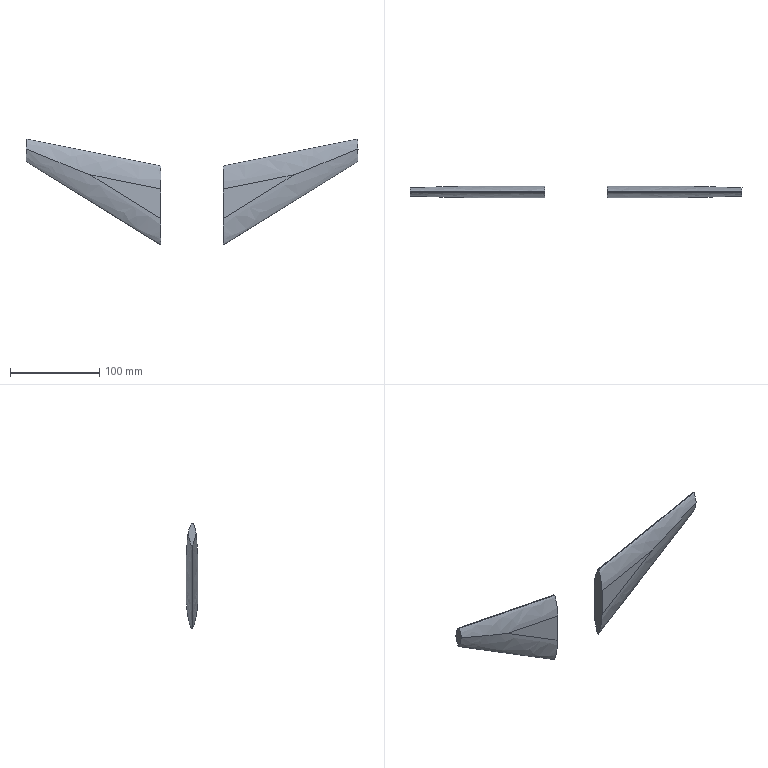Part | SolidWorks | features Fillet 4, Extrusion 1, MirrorSolid 1 | 2 solids | 18 faces | box 372.694 x 12.7 x 118.906 mm | volume 155010 mm3 | plane 10 | spline 8